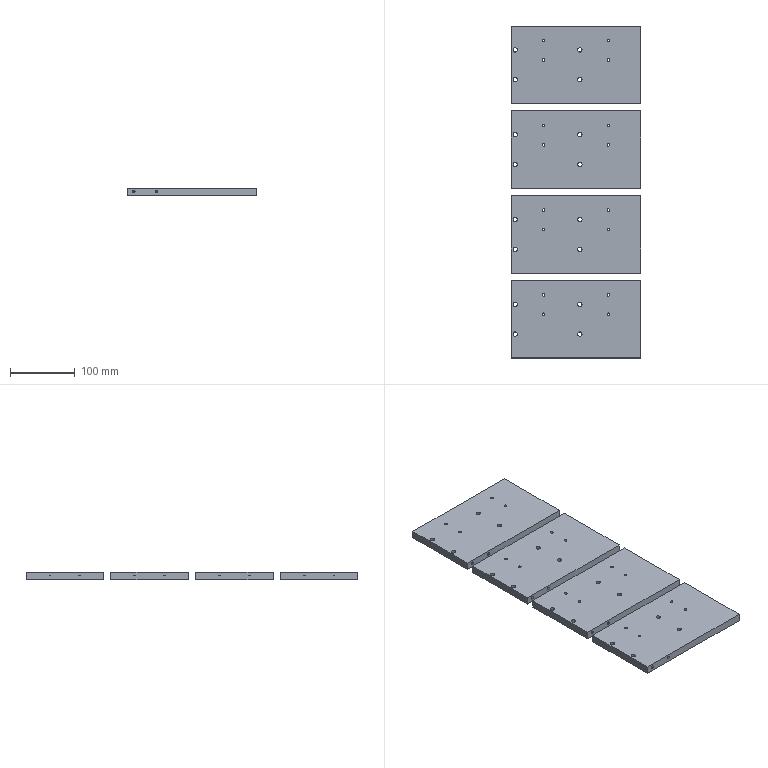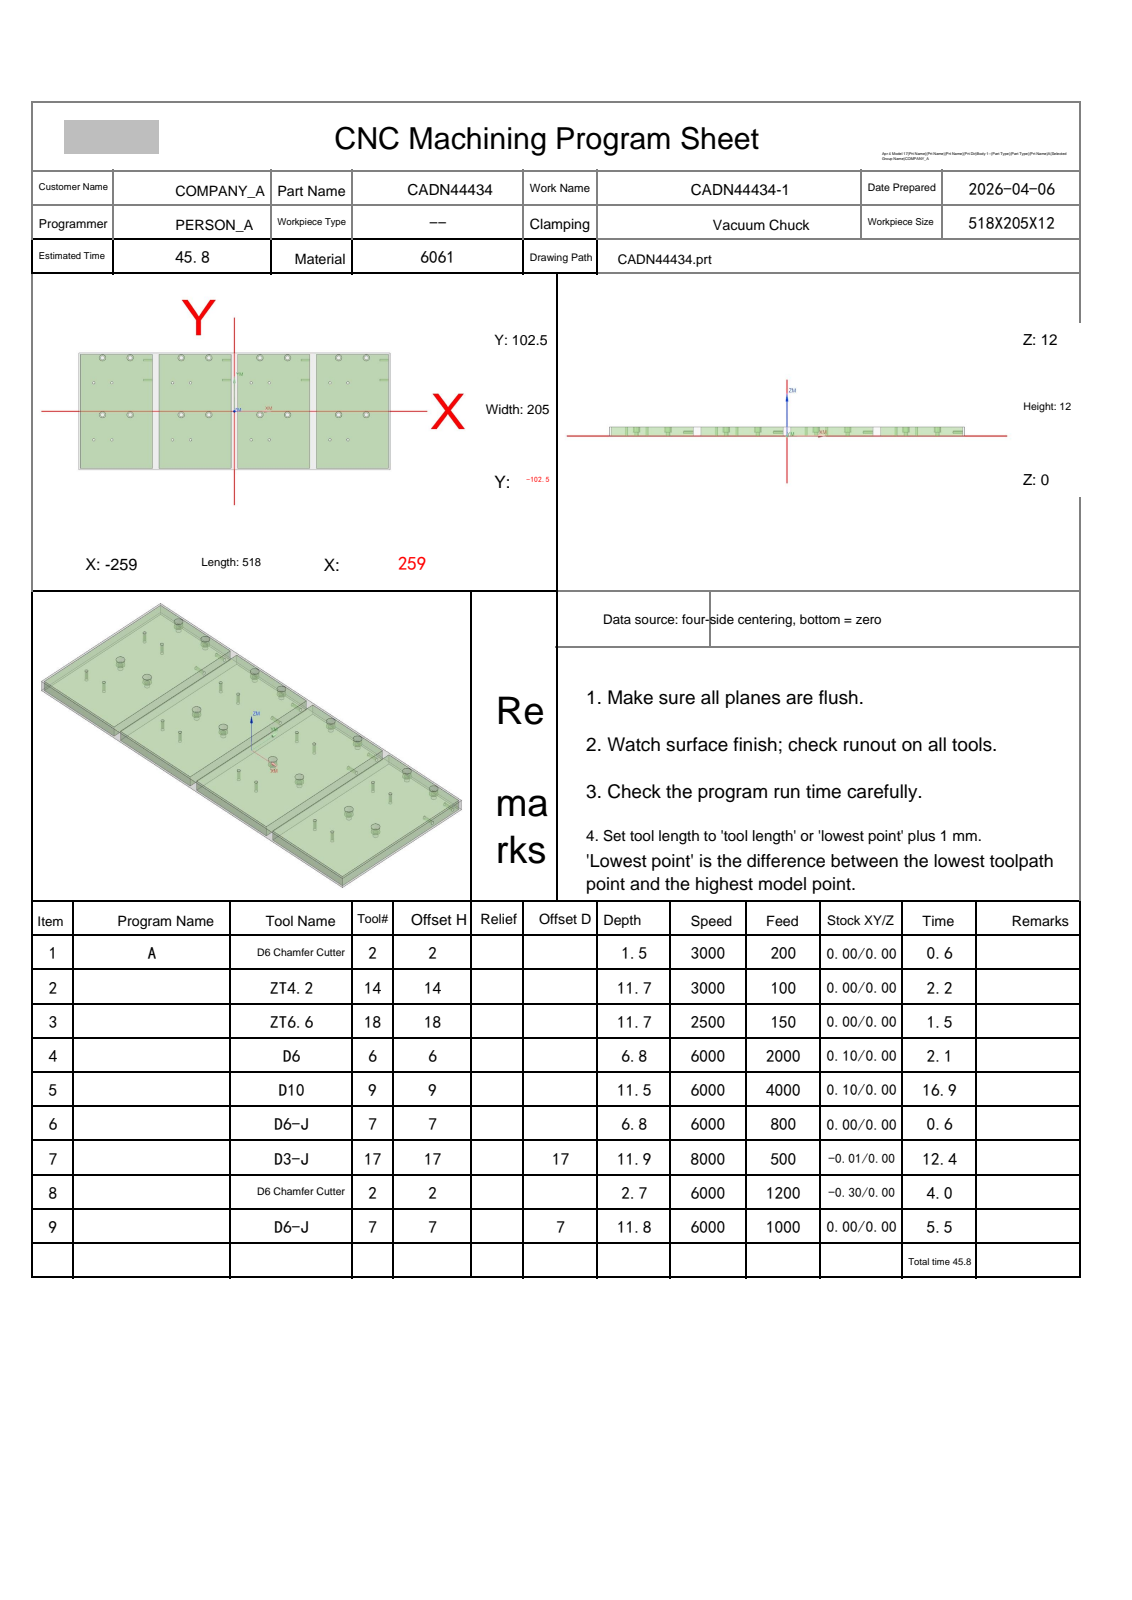NC program | NX | posted by the shop | part box 200 x 513 x 12 mm
Lines 1644 to 2457 of 7719:
N7 T17 M06
(D3-J  D=3. R=0. H=17 ce=-0.01 di=0.00)
G00 G90 G54 X28.521 Y-50.146 M03 S8000
G43 H17 Z32.
M08
Z12.5
G01 X28.543 Y-50.074 Z12.496 F500.
Y-49.926 Z12.488
X28.491 Y-49.757 Z12.479
X28.387 Y-49.613 Z12.47
X28.243 Y-49.509 Z12.46
X28.074 Y-49.457 Z12.451
X27.926 Z12.443
X27.757 Y-49.509 Z12.434
X27.613 Y-49.613 Z12.425
X27.509 Y-49.757 Z12.416
X27.457 Y-49.926 Z12.406
Y-50.074 Z12.398
X27.505 Y-50.235 Z12.39
X27.6 Y-50.375 Z12.381
X27.733 Y-50.478 Z12.372
X27.891 Y-50.537 Z12.363
X28.074 Y-50.543 Z12.354
X28.243 Y-50.491 Z12.344
X28.387 Y-50.387 Z12.335
X28.491 Y-50.243 Z12.326
X28.543 Y-50.074 Z12.316
Y-49.926 Z12.309
X28.491 Y-49.757 Z12.299
X28.387 Y-49.613 Z12.29
X28.243 Y-49.509 Z12.281
X28.074 Y-49.457 Z12.271
X27.926 Z12.264
X27.757 Y-49.509 Z12.254
X27.613 Y-49.613 Z12.245
X27.509 Y-49.757 Z12.236
X27.457 Y-49.926 Z12.227
Y-50.074 Z12.219
X27.505 Y-50.235 Z12.21
X27.6 Y-50.375 Z12.201
X27.733 Y-50.478 Z12.192
X27.891 Y-50.537 Z12.184
X28.074 Y-50.543 Z12.174
X28.243 Y-50.491 Z12.165
X28.387 Y-50.387 Z12.155
X28.491 Y-50.243 Z12.146
X28.543 Y-50.074 Z12.137
Y-49.926 Z12.129
X28.491 Y-49.757 Z12.12
X28.387 Y-49.613 Z12.11
X28.243 Y-49.509 Z12.101
X28.074 Y-49.457 Z12.092
X27.926 Z12.084
X27.757 Y-49.509 Z12.075
X27.613 Y-49.613 Z12.066
X27.509 Y-49.757 Z12.056
X27.457 Y-49.926 Z12.047
Y-50.074 Z12.039
X27.505 Y-50.235 Z12.03
X27.6 Y-50.375 Z12.022
X27.733 Y-50.478 Z12.013
X27.891 Y-50.537 Z12.004
X27.965 Y-50.542 Z12.
G41 D17
X28. Y-50.577
G03 X28.577 Y-50. Z11.926 I0.0 J.577
X28. Y-49.423 Z11.852 I-.577 J0.0
X27.423 Y-50. Z11.778 I0.0 J-.577
X28. Y-50.577 Z11.704 I.577 J0.0
X28.577 Y-50. Z11.63 I0.0 J.577
X28. Y-49.423 Z11.556 I-.577 J0.0
X27.423 Y-50. Z11.482 I0.0 J-.577
X28. Y-50.577 Z11.408 I.577 J0.0
X28.577 Y-50. Z11.333 I0.0 J.577
X28. Y-49.423 Z11.259 I-.577 J0.0
X27.423 Y-50. Z11.185 I0.0 J-.577
X28. Y-50.577 Z11.111 I.577 J0.0
X28.577 Y-50. Z11.037 I0.0 J.577
X28. Y-49.423 Z10.963 I-.577 J0.0
X27.423 Y-50. Z10.889 I0.0 J-.577
X28. Y-50.577 Z10.815 I.577 J0.0
X28.577 Y-50. Z10.741 I0.0 J.577
X28. Y-49.423 Z10.667 I-.577 J0.0
X27.423 Y-50. Z10.593 I0.0 J-.577
X28. Y-50.577 Z10.519 I.577 J0.0
X28.577 Y-50. Z10.445 I0.0 J.577
X28. Y-49.423 Z10.371 I-.577 J0.0
X27.423 Y-50. Z10.297 I0.0 J-.577
X28. Y-50.577 Z10.223 I.577 J0.0
X28.577 Y-50. Z10.148 I0.0 J.577
X28. Y-49.423 Z10.074 I-.577 J0.0
X27.423 Y-50. Z10. I0.0 J-.577
X28. Y-50.577 Z9.926 I.577 J0.0
X28.577 Y-50. Z9.852 I0.0 J.577
X28. Y-49.423 Z9.778 I-.577 J0.0
X27.423 Y-50. Z9.704 I0.0 J-.577
X28. Y-50.577 Z9.63 I.577 J0.0
X28.577 Y-50. Z9.556 I0.0 J.577
X28. Y-49.423 Z9.482 I-.577 J0.0
X27.423 Y-50. Z9.408 I0.0 J-.577
X28. Y-50.577 Z9.334 I.577 J0.0
X28.577 Y-50. Z9.26 I0.0 J.577
X28. Y-49.423 Z9.186 I-.577 J0.0
X27.423 Y-50. Z9.112 I0.0 J-.577
X28. Y-50.577 Z9.038 I.577 J0.0
X28.577 Y-50. Z8.963 I0.0 J.577
X28. Y-49.423 Z8.889 I-.577 J0.0
X27.423 Y-50. Z8.815 I0.0 J-.577
X28. Y-50.577 Z8.741 I.577 J0.0
X28.577 Y-50. Z8.667 I0.0 J.577
X28. Y-49.423 Z8.593 I-.577 J0.0
X27.423 Y-50. Z8.519 I0.0 J-.577
X28. Y-50.577 Z8.445 I.577 J0.0
X28.577 Y-50. Z8.371 I0.0 J.577
X28. Y-49.423 Z8.297 I-.577 J0.0
X27.423 Y-50. Z8.223 I0.0 J-.577
X28. Y-50.577 Z8.149 I.577 J0.0
X28.577 Y-50. Z8.075 I0.0 J.577
X28. Y-49.423 Z8.001 I-.577 J0.0
X27.423 Y-50. Z7.927 I0.0 J-.577
X28. Y-50.577 Z7.853 I.577 J0.0
X28.577 Y-50. Z7.778 I0.0 J.577
X28. Y-49.423 Z7.704 I-.577 J0.0
X27.423 Y-50. Z7.63 I0.0 J-.577
X28. Y-50.577 Z7.556 I.577 J0.0
X28.577 Y-50. Z7.482 I0.0 J.577
X28. Y-49.423 Z7.408 I-.577 J0.0
X27.423 Y-50. Z7.334 I0.0 J-.577
X28. Y-50.577 Z7.26 I.577 J0.0
X28.577 Y-50. Z7.186 I0.0 J.577
X28. Y-49.423 Z7.112 I-.577 J0.0
X27.423 Y-50. Z7.038 I0.0 J-.577
X28. Y-50.577 Z6.964 I.577 J0.0
X28.577 Y-50. Z6.89 I0.0 J.577
X28. Y-49.423 Z6.816 I-.577 J0.0
X27.423 Y-50. Z6.742 I0.0 J-.577
X28. Y-50.577 Z6.668 I.577 J0.0
X28.577 Y-50. Z6.593 I0.0 J.577
X28. Y-49.423 Z6.519 I-.577 J0.0
X27.423 Y-50. Z6.445 I0.0 J-.577
X28. Y-50.577 Z6.371 I.577 J0.0
X28.577 Y-50. Z6.297 I0.0 J.577
X28. Y-49.423 Z6.223 I-.577 J0.0
X27.423 Y-50. Z6.149 I0.0 J-.577
X28. Y-50.577 Z6.075 I.577 J0.0
X28.577 Y-50. Z6.001 I0.0 J.577
X28. Y-49.423 Z5.927 I-.577 J0.0
X27.423 Y-50. Z5.853 I0.0 J-.577
X28. Y-50.577 Z5.779 I.577 J0.0
X28.577 Y-50. Z5.705 I0.0 J.577
X28. Y-49.423 Z5.631 I-.577 J0.0
X27.423 Y-50. Z5.557 I0.0 J-.577
X28. Y-50.577 Z5.483 I.577 J0.0
X28.577 Y-50. Z5.408 I0.0 J.577
X28. Y-49.423 Z5.334 I-.577 J0.0
X27.423 Y-50. Z5.26 I0.0 J-.577
X28. Y-50.577 Z5.186 I.577 J0.0
X28.577 Y-50. Z5.112 I0.0 J.577
X28. Y-49.423 Z5.038 I-.577 J0.0
X27.423 Y-50. Z4.964 I0.0 J-.577
X28. Y-50.577 Z4.89 I.577 J0.0
X28.577 Y-50. Z4.816 I0.0 J.577
X28. Y-49.423 Z4.742 I-.577 J0.0
X27.423 Y-50. Z4.668 I0.0 J-.577
X28. Y-50.577 Z4.594 I.577 J0.0
X28.577 Y-50. Z4.52 I0.0 J.577
X28. Y-49.423 Z4.446 I-.577 J0.0
X27.423 Y-50. Z4.372 I0.0 J-.577
X28. Y-50.577 Z4.298 I.577 J0.0
X28.577 Y-50. Z4.223 I0.0 J.577
X28. Y-49.423 Z4.149 I-.577 J0.0
X27.423 Y-50. Z4.075 I0.0 J-.577
X28. Y-50.577 Z4.001 I.577 J0.0
X28.577 Y-50. Z3.927 I0.0 J.577
X28. Y-49.423 Z3.853 I-.577 J0.0
X27.423 Y-50. Z3.779 I0.0 J-.577
X28. Y-50.577 Z3.705 I.577 J0.0
X28.577 Y-50. Z3.631 I0.0 J.577
X28. Y-49.423 Z3.557 I-.577 J0.0
X27.423 Y-50. Z3.483 I0.0 J-.577
X28. Y-50.577 Z3.409 I.577 J0.0
X28.577 Y-50. Z3.335 I0.0 J.577
X28. Y-49.423 Z3.261 I-.577 J0.0
X27.423 Y-50. Z3.187 I0.0 J-.577
X28. Y-50.577 Z3.113 I.577 J0.0
X28.577 Y-50. Z3.038 I0.0 J.577
X28. Y-49.423 Z2.964 I-.577 J0.0
X27.423 Y-50. Z2.89 I0.0 J-.577
X28. Y-50.577 Z2.816 I.577 J0.0
X28.577 Y-50. Z2.742 I0.0 J.577
X28. Y-49.423 Z2.668 I-.577 J0.0
X27.423 Y-50. Z2.594 I0.0 J-.577
X28. Y-50.577 Z2.52 I.577 J0.0
X28.577 Y-50. Z2.446 I0.0 J.577
X28. Y-49.423 Z2.372 I-.577 J0.0
X27.423 Y-50. Z2.298 I0.0 J-.577
X28. Y-50.577 Z2.224 I.577 J0.0
X28.577 Y-50. Z2.15 I0.0 J.577
X28. Y-49.423 Z2.076 I-.577 J0.0
X27.423 Y-50. Z2.002 I0.0 J-.577
X28. Y-50.577 Z1.928 I.577 J0.0
X28.577 Y-50. Z1.853 I0.0 J.577
X28. Y-49.423 Z1.779 I-.577 J0.0
X27.423 Y-50. Z1.705 I0.0 J-.577
X28. Y-50.577 Z1.631 I.577 J0.0
X28.577 Y-50. Z1.557 I0.0 J.577
X28. Y-49.423 Z1.483 I-.577 J0.0
X27.423 Y-50. Z1.409 I0.0 J-.577
X28. Y-50.577 Z1.335 I.577 J0.0
X28.577 Y-50. Z1.261 I0.0 J.577
X28. Y-49.423 Z1.187 I-.577 J0.0
X27.423 Y-50. Z1.113 I0.0 J-.577
X28. Y-50.577 Z1.039 I.577 J0.0
X28.577 Y-50. Z.965 I0.0 J.577
X28. Y-49.423 Z.891 I-.577 J0.0
X27.423 Y-50. Z.817 I0.0 J-.577
X28. Y-50.577 Z.743 I.577 J0.0
X28.577 Y-50. Z.668 I0.0 J.577
X28. Y-49.423 Z.594 I-.577 J0.0
X27.423 Y-50. Z.52 I0.0 J-.577
X28. Y-50.577 Z.446 I.577 J0.0
X28.577 Y-50. Z.372 I0.0 J.577
X28. Y-49.423 Z.298 I-.577 J0.0
X27.423 Y-50. Z.224 I0.0 J-.577
X28. Y-50.577 Z.15 I.577 J0.0
X28.577 Y-50. I0.0 J.577
X28. Y-49.423 I-.577 J0.0
X27.423 Y-50. I0.0 J-.577
X28. Y-50.577 I.577 J0.0
X28.369 Y-50.444 I0.0 J.577
G01 X28.388 Y-50.424
X28.391 Y-50.396
X28.375 Y-50.373
G40 X28.343 Y-50.335
Z1.15
G00 Z32.
X58.521 Y-50.146
Z12.5
G01 X58.543 Y-50.074 Z12.496
Y-49.926 Z12.488
X58.491 Y-49.757 Z12.479
X58.387 Y-49.613 Z12.47
X58.243 Y-49.509 Z12.46
X58.074 Y-49.457 Z12.451
X57.926 Z12.443
X57.757 Y-49.509 Z12.434
X57.613 Y-49.613 Z12.425
X57.509 Y-49.757 Z12.416
X57.457 Y-49.926 Z12.406
Y-50.074 Z12.398
X57.505 Y-50.235 Z12.39
X57.6 Y-50.375 Z12.381
X57.733 Y-50.478 Z12.372
X57.891 Y-50.537 Z12.363
X58.074 Y-50.543 Z12.354
X58.243 Y-50.491 Z12.344
X58.387 Y-50.387 Z12.335
X58.491 Y-50.243 Z12.326
X58.543 Y-50.074 Z12.316
Y-49.926 Z12.309
X58.491 Y-49.757 Z12.299
X58.387 Y-49.613 Z12.29
X58.243 Y-49.509 Z12.281
X58.074 Y-49.457 Z12.271
X57.926 Z12.264
X57.757 Y-49.509 Z12.254
X57.613 Y-49.613 Z12.245
X57.509 Y-49.757 Z12.236
X57.457 Y-49.926 Z12.227
Y-50.074 Z12.219
X57.505 Y-50.235 Z12.21
X57.6 Y-50.375 Z12.201
X57.733 Y-50.478 Z12.192
X57.891 Y-50.537 Z12.184
X58.074 Y-50.543 Z12.174
X58.243 Y-50.491 Z12.165
X58.387 Y-50.387 Z12.155
X58.491 Y-50.243 Z12.146
X58.543 Y-50.074 Z12.137
Y-49.926 Z12.129
X58.491 Y-49.757 Z12.12
X58.387 Y-49.613 Z12.11
X58.243 Y-49.509 Z12.101
X58.074 Y-49.457 Z12.092
X57.926 Z12.084
X57.757 Y-49.509 Z12.075
X57.613 Y-49.613 Z12.066
X57.509 Y-49.757 Z12.056
X57.457 Y-49.926 Z12.047
Y-50.074 Z12.039
X57.505 Y-50.235 Z12.03
X57.6 Y-50.375 Z12.022
X57.733 Y-50.478 Z12.013
X57.891 Y-50.537 Z12.004
X57.965 Y-50.542 Z12.
G41 D17
X58. Y-50.577
G03 X58.577 Y-50. Z11.926 I0.0 J.577
X58. Y-49.423 Z11.852 I-.577 J0.0
X57.423 Y-50. Z11.778 I0.0 J-.577
X58. Y-50.577 Z11.704 I.577 J0.0
X58.577 Y-50. Z11.63 I0.0 J.577
X58. Y-49.423 Z11.556 I-.577 J0.0
X57.423 Y-50. Z11.482 I0.0 J-.577
X58. Y-50.577 Z11.408 I.577 J0.0
X58.577 Y-50. Z11.333 I0.0 J.577
X58. Y-49.423 Z11.259 I-.577 J0.0
X57.423 Y-50. Z11.185 I0.0 J-.577
X58. Y-50.577 Z11.111 I.577 J0.0
X58.577 Y-50. Z11.037 I0.0 J.577
X58. Y-49.423 Z10.963 I-.577 J0.0
X57.423 Y-50. Z10.889 I0.0 J-.577
X58. Y-50.577 Z10.815 I.577 J0.0
X58.577 Y-50. Z10.741 I0.0 J.577
X58. Y-49.423 Z10.667 I-.577 J0.0
X57.423 Y-50. Z10.593 I0.0 J-.577
X58. Y-50.577 Z10.519 I.577 J0.0
X58.577 Y-50. Z10.445 I0.0 J.577
X58. Y-49.423 Z10.371 I-.577 J0.0
X57.423 Y-50. Z10.297 I0.0 J-.577
X58. Y-50.577 Z10.223 I.577 J0.0
X58.577 Y-50. Z10.148 I0.0 J.577
X58. Y-49.423 Z10.074 I-.577 J0.0
X57.423 Y-50. Z10. I0.0 J-.577
X58. Y-50.577 Z9.926 I.577 J0.0
X58.577 Y-50. Z9.852 I0.0 J.577
X58. Y-49.423 Z9.778 I-.577 J0.0
X57.423 Y-50. Z9.704 I0.0 J-.577
X58. Y-50.577 Z9.63 I.577 J0.0
X58.577 Y-50. Z9.556 I0.0 J.577
X58. Y-49.423 Z9.482 I-.577 J0.0
X57.423 Y-50. Z9.408 I0.0 J-.577
X58. Y-50.577 Z9.334 I.577 J0.0
X58.577 Y-50. Z9.26 I0.0 J.577
X58. Y-49.423 Z9.186 I-.577 J0.0
X57.423 Y-50. Z9.112 I0.0 J-.577
X58. Y-50.577 Z9.038 I.577 J0.0
X58.577 Y-50. Z8.963 I0.0 J.577
X58. Y-49.423 Z8.889 I-.577 J0.0
X57.423 Y-50. Z8.815 I0.0 J-.577
X58. Y-50.577 Z8.741 I.577 J0.0
X58.577 Y-50. Z8.667 I0.0 J.577
X58. Y-49.423 Z8.593 I-.577 J0.0
X57.423 Y-50. Z8.519 I0.0 J-.577
X58. Y-50.577 Z8.445 I.577 J0.0
X58.577 Y-50. Z8.371 I0.0 J.577
X58. Y-49.423 Z8.297 I-.577 J0.0
X57.423 Y-50. Z8.223 I0.0 J-.577
X58. Y-50.577 Z8.149 I.577 J0.0
X58.577 Y-50. Z8.075 I0.0 J.577
X58. Y-49.423 Z8.001 I-.577 J0.0
X57.423 Y-50. Z7.927 I0.0 J-.577
X58. Y-50.577 Z7.853 I.577 J0.0
X58.577 Y-50. Z7.778 I0.0 J.577
X58. Y-49.423 Z7.704 I-.577 J0.0
X57.423 Y-50. Z7.63 I0.0 J-.577
X58. Y-50.577 Z7.556 I.577 J0.0
X58.577 Y-50. Z7.482 I0.0 J.577
X58. Y-49.423 Z7.408 I-.577 J0.0
X57.423 Y-50. Z7.334 I0.0 J-.577
X58. Y-50.577 Z7.26 I.577 J0.0
X58.577 Y-50. Z7.186 I0.0 J.577
X58. Y-49.423 Z7.112 I-.577 J0.0
X57.423 Y-50. Z7.038 I0.0 J-.577
X58. Y-50.577 Z6.964 I.577 J0.0
X58.577 Y-50. Z6.89 I0.0 J.577
X58. Y-49.423 Z6.816 I-.577 J0.0
X57.423 Y-50. Z6.742 I0.0 J-.577
X58. Y-50.577 Z6.668 I.577 J0.0
X58.577 Y-50. Z6.593 I0.0 J.577
X58. Y-49.423 Z6.519 I-.577 J0.0
X57.423 Y-50. Z6.445 I0.0 J-.577
X58. Y-50.577 Z6.371 I.577 J0.0
X58.577 Y-50. Z6.297 I0.0 J.577
X58. Y-49.423 Z6.223 I-.577 J0.0
X57.423 Y-50. Z6.149 I0.0 J-.577
X58. Y-50.577 Z6.075 I.577 J0.0
X58.577 Y-50. Z6.001 I0.0 J.577
X58. Y-49.423 Z5.927 I-.577 J0.0
X57.423 Y-50. Z5.853 I0.0 J-.577
X58. Y-50.577 Z5.779 I.577 J0.0
X58.577 Y-50. Z5.705 I0.0 J.577
X58. Y-49.423 Z5.631 I-.577 J0.0
X57.423 Y-50. Z5.557 I0.0 J-.577
X58. Y-50.577 Z5.483 I.577 J0.0
X58.577 Y-50. Z5.408 I0.0 J.577
X58. Y-49.423 Z5.334 I-.577 J0.0
X57.423 Y-50. Z5.26 I0.0 J-.577
X58. Y-50.577 Z5.186 I.577 J0.0
X58.577 Y-50. Z5.112 I0.0 J.577
X58. Y-49.423 Z5.038 I-.577 J0.0
X57.423 Y-50. Z4.964 I0.0 J-.577
X58. Y-50.577 Z4.89 I.577 J0.0
X58.577 Y-50. Z4.816 I0.0 J.577
X58. Y-49.423 Z4.742 I-.577 J0.0
X57.423 Y-50. Z4.668 I0.0 J-.577
X58. Y-50.577 Z4.594 I.577 J0.0
X58.577 Y-50. Z4.52 I0.0 J.577
X58. Y-49.423 Z4.446 I-.577 J0.0
X57.423 Y-50. Z4.372 I0.0 J-.577
X58. Y-50.577 Z4.298 I.577 J0.0
X58.577 Y-50. Z4.223 I0.0 J.577
X58. Y-49.423 Z4.149 I-.577 J0.0
X57.423 Y-50. Z4.075 I0.0 J-.577
X58. Y-50.577 Z4.001 I.577 J0.0
X58.577 Y-50. Z3.927 I0.0 J.577
X58. Y-49.423 Z3.853 I-.577 J0.0
X57.423 Y-50. Z3.779 I0.0 J-.577
X58. Y-50.577 Z3.705 I.577 J0.0
X58.577 Y-50. Z3.631 I0.0 J.577
X58. Y-49.423 Z3.557 I-.577 J0.0
X57.423 Y-50. Z3.483 I0.0 J-.577
X58. Y-50.577 Z3.409 I.577 J0.0
X58.577 Y-50. Z3.335 I0.0 J.577
X58. Y-49.423 Z3.261 I-.577 J0.0
X57.423 Y-50. Z3.187 I0.0 J-.577
X58. Y-50.577 Z3.113 I.577 J0.0
X58.577 Y-50. Z3.038 I0.0 J.577
X58. Y-49.423 Z2.964 I-.577 J0.0
X57.423 Y-50. Z2.89 I0.0 J-.577
X58. Y-50.577 Z2.816 I.577 J0.0
X58.577 Y-50. Z2.742 I0.0 J.577
X58. Y-49.423 Z2.668 I-.577 J0.0
X57.423 Y-50. Z2.594 I0.0 J-.577
X58. Y-50.577 Z2.52 I.577 J0.0
X58.577 Y-50. Z2.446 I0.0 J.577
X58. Y-49.423 Z2.372 I-.577 J0.0
X57.423 Y-50. Z2.298 I0.0 J-.577
X58. Y-50.577 Z2.224 I.577 J0.0
X58.577 Y-50. Z2.15 I0.0 J.577
X58. Y-49.423 Z2.076 I-.577 J0.0
X57.423 Y-50. Z2.002 I0.0 J-.577
X58. Y-50.577 Z1.928 I.577 J0.0
X58.577 Y-50. Z1.853 I0.0 J.577
X58. Y-49.423 Z1.779 I-.577 J0.0
X57.423 Y-50. Z1.705 I0.0 J-.577
X58. Y-50.577 Z1.631 I.577 J0.0
X58.577 Y-50. Z1.557 I0.0 J.577
X58. Y-49.423 Z1.483 I-.577 J0.0
X57.423 Y-50. Z1.409 I0.0 J-.577
X58. Y-50.577 Z1.335 I.577 J0.0
X58.577 Y-50. Z1.261 I0.0 J.577
X58. Y-49.423 Z1.187 I-.577 J0.0
X57.423 Y-50. Z1.113 I0.0 J-.577
X58. Y-50.577 Z1.039 I.577 J0.0
X58.577 Y-50. Z.965 I0.0 J.577
X58. Y-49.423 Z.891 I-.577 J0.0
X57.423 Y-50. Z.817 I0.0 J-.577
X58. Y-50.577 Z.743 I.577 J0.0
X58.577 Y-50. Z.668 I0.0 J.577
X58. Y-49.423 Z.594 I-.577 J0.0
X57.423 Y-50. Z.52 I0.0 J-.577
X58. Y-50.577 Z.446 I.577 J0.0
X58.577 Y-50. Z.372 I0.0 J.577
X58. Y-49.423 Z.298 I-.577 J0.0
X57.423 Y-50. Z.224 I0.0 J-.577
X58. Y-50.577 Z.15 I.577 J0.0
X58.577 Y-50. I0.0 J.577
X58. Y-49.423 I-.577 J0.0
X57.423 Y-50. I0.0 J-.577
X58. Y-50.577 I.577 J0.0
X58.369 Y-50.444 I0.0 J.577
G01 X58.388 Y-50.424
X58.391 Y-50.396
X58.375 Y-50.373
G40 X58.343 Y-50.335
Z1.15
G00 Z32.
X159.521 Y-50.146
Z12.5
G01 X159.543 Y-50.074 Z12.496
Y-49.926 Z12.488
X159.491 Y-49.757 Z12.479
X159.387 Y-49.613 Z12.47
X159.243 Y-49.509 Z12.46
X159.074 Y-49.457 Z12.451
X158.926 Z12.443
X158.757 Y-49.509 Z12.434
X158.613 Y-49.613 Z12.425
X158.509 Y-49.757 Z12.416
X158.457 Y-49.926 Z12.406
Y-50.074 Z12.398
X158.505 Y-50.235 Z12.39
X158.6 Y-50.375 Z12.381
X158.733 Y-50.478 Z12.372
X158.891 Y-50.537 Z12.363
X159.074 Y-50.543 Z12.354
X159.243 Y-50.491 Z12.344
X159.387 Y-50.387 Z12.335
X159.491 Y-50.243 Z12.326
X159.543 Y-50.074 Z12.316
Y-49.926 Z12.309
X159.491 Y-49.757 Z12.299
X159.387 Y-49.613 Z12.29
X159.243 Y-49.509 Z12.281
X159.074 Y-49.457 Z12.271
X158.926 Z12.264
X158.757 Y-49.509 Z12.254
X158.613 Y-49.613 Z12.245
X158.509 Y-49.757 Z12.236
X158.457 Y-49.926 Z12.227
Y-50.074 Z12.219
X158.505 Y-50.235 Z12.21
X158.6 Y-50.375 Z12.201
X158.733 Y-50.478 Z12.192
X158.891 Y-50.537 Z12.184
X159.074 Y-50.543 Z12.174
X159.243 Y-50.491 Z12.165
X159.387 Y-50.387 Z12.155
X159.491 Y-50.243 Z12.146
X159.543 Y-50.074 Z12.137
Y-49.926 Z12.129
X159.491 Y-49.757 Z12.12
X159.387 Y-49.613 Z12.11
X159.243 Y-49.509 Z12.101
X159.074 Y-49.457 Z12.092
X158.926 Z12.084
X158.757 Y-49.509 Z12.075
X158.613 Y-49.613 Z12.066
X158.509 Y-49.757 Z12.056
X158.457 Y-49.926 Z12.047
Y-50.074 Z12.039
X158.505 Y-50.235 Z12.03
X158.6 Y-50.375 Z12.022
X158.733 Y-50.478 Z12.013
X158.891 Y-50.537 Z12.004
X158.965 Y-50.542 Z12.
G41 D17
X159. Y-50.577
G03 X159.577 Y-50. Z11.926 I0.0 J.577
X159. Y-49.423 Z11.852 I-.577 J0.0
X158.423 Y-50. Z11.778 I0.0 J-.577
X159. Y-50.577 Z11.704 I.577 J0.0
X159.577 Y-50. Z11.63 I0.0 J.577
X159. Y-49.423 Z11.556 I-.577 J0.0
X158.423 Y-50. Z11.482 I0.0 J-.577
X159. Y-50.577 Z11.408 I.577 J0.0
X159.577 Y-50. Z11.333 I0.0 J.577
X159. Y-49.423 Z11.259 I-.577 J0.0
X158.423 Y-50. Z11.185 I0.0 J-.577
X159. Y-50.577 Z11.111 I.577 J0.0
X159.577 Y-50. Z11.037 I0.0 J.577
X159. Y-49.423 Z10.963 I-.577 J0.0
X158.423 Y-50. Z10.889 I0.0 J-.577
X159. Y-50.577 Z10.815 I.577 J0.0
X159.577 Y-50. Z10.741 I0.0 J.577
X159. Y-49.423 Z10.667 I-.577 J0.0
X158.423 Y-50. Z10.593 I0.0 J-.577
X159. Y-50.577 Z10.519 I.577 J0.0
X159.577 Y-50. Z10.445 I0.0 J.577
X159. Y-49.423 Z10.371 I-.577 J0.0
X158.423 Y-50. Z10.297 I0.0 J-.577
X159. Y-50.577 Z10.223 I.577 J0.0
X159.577 Y-50. Z10.148 I0.0 J.577
X159. Y-49.423 Z10.074 I-.577 J0.0
X158.423 Y-50. Z10. I0.0 J-.577
X159. Y-50.577 Z9.926 I.577 J0.0
X159.577 Y-50. Z9.852 I0.0 J.577
X159. Y-49.423 Z9.778 I-.577 J0.0
X158.423 Y-50. Z9.704 I0.0 J-.577
X159. Y-50.577 Z9.63 I.577 J0.0
X159.577 Y-50. Z9.556 I0.0 J.577
X159. Y-49.423 Z9.482 I-.577 J0.0
X158.423 Y-50. Z9.408 I0.0 J-.577
X159. Y-50.577 Z9.334 I.577 J0.0
X159.577 Y-50. Z9.26 I0.0 J.577
X159. Y-49.423 Z9.186 I-.577 J0.0
X158.423 Y-50. Z9.112 I0.0 J-.577
X159. Y-50.577 Z9.038 I.577 J0.0
X159.577 Y-50. Z8.963 I0.0 J.577
X159. Y-49.423 Z8.889 I-.577 J0.0
X158.423 Y-50. Z8.815 I0.0 J-.577
X159. Y-50.577 Z8.741 I.577 J0.0
X159.577 Y-50. Z8.667 I0.0 J.577
X159. Y-49.423 Z8.593 I-.577 J0.0
X158.423 Y-50. Z8.519 I0.0 J-.577
X159. Y-50.577 Z8.445 I.577 J0.0
X159.577 Y-50. Z8.371 I0.0 J.577
X159. Y-49.423 Z8.297 I-.577 J0.0
X158.423 Y-50. Z8.223 I0.0 J-.577
X159. Y-50.577 Z8.149 I.577 J0.0
X159.577 Y-50. Z8.075 I0.0 J.577
X159. Y-49.423 Z8.001 I-.577 J0.0
X158.423 Y-50. Z7.927 I0.0 J-.577
X159. Y-50.577 Z7.853 I.577 J0.0
X159.577 Y-50. Z7.778 I0.0 J.577
X159. Y-49.423 Z7.704 I-.577 J0.0
X158.423 Y-50. Z7.63 I0.0 J-.577
X159. Y-50.577 Z7.556 I.577 J0.0
X159.577 Y-50. Z7.482 I0.0 J.577
X159. Y-49.423 Z7.408 I-.577 J0.0
X158.423 Y-50. Z7.334 I0.0 J-.577
X159. Y-50.577 Z7.26 I.577 J0.0
X159.577 Y-50. Z7.186 I0.0 J.577
X159. Y-49.423 Z7.112 I-.577 J0.0
X158.423 Y-50. Z7.038 I0.0 J-.577
X159. Y-50.577 Z6.964 I.577 J0.0
X159.577 Y-50. Z6.89 I0.0 J.577
X159. Y-49.423 Z6.816 I-.577 J0.0
X158.423 Y-50. Z6.742 I0.0 J-.577
X159. Y-50.577 Z6.668 I.577 J0.0
X159.577 Y-50. Z6.593 I0.0 J.577
X159. Y-49.423 Z6.519 I-.577 J0.0
X158.423 Y-50. Z6.445 I0.0 J-.577
X159. Y-50.577 Z6.371 I.577 J0.0
X159.577 Y-50. Z6.297 I0.0 J.577
X159. Y-49.423 Z6.223 I-.577 J0.0
X158.423 Y-50. Z6.149 I0.0 J-.577
X159. Y-50.577 Z6.075 I.577 J0.0
X159.577 Y-50. Z6.001 I0.0 J.577
X159. Y-49.423 Z5.927 I-.577 J0.0
X158.423 Y-50. Z5.853 I0.0 J-.577
X159. Y-50.577 Z5.779 I.577 J0.0
X159.577 Y-50. Z5.705 I0.0 J.577
X159. Y-49.423 Z5.631 I-.577 J0.0
X158.423 Y-50. Z5.557 I0.0 J-.577
X159. Y-50.577 Z5.483 I.577 J0.0
X159.577 Y-50. Z5.408 I0.0 J.577
X159. Y-49.423 Z5.334 I-.577 J0.0
X158.423 Y-50. Z5.26 I0.0 J-.577
X159. Y-50.577 Z5.186 I.577 J0.0
X159.577 Y-50. Z5.112 I0.0 J.577
X159. Y-49.423 Z5.038 I-.577 J0.0
X158.423 Y-50. Z4.964 I0.0 J-.577
X159. Y-50.577 Z4.89 I.577 J0.0
X159.577 Y-50. Z4.816 I0.0 J.577
X159. Y-49.423 Z4.742 I-.577 J0.0
X158.423 Y-50. Z4.668 I0.0 J-.577
X159. Y-50.577 Z4.594 I.577 J0.0
X159.577 Y-50. Z4.52 I0.0 J.577
X159. Y-49.423 Z4.446 I-.577 J0.0
X158.423 Y-50. Z4.372 I0.0 J-.577
X159. Y-50.577 Z4.298 I.577 J0.0
X159.577 Y-50. Z4.223 I0.0 J.577
X159. Y-49.423 Z4.149 I-.577 J0.0
X158.423 Y-50. Z4.075 I0.0 J-.577
X159. Y-50.577 Z4.001 I.577 J0.0
X159.577 Y-50. Z3.927 I0.0 J.577
X159. Y-49.423 Z3.853 I-.577 J0.0
X158.423 Y-50. Z3.779 I0.0 J-.577
X159. Y-50.577 Z3.705 I.577 J0.0
X159.577 Y-50. Z3.631 I0.0 J.577
X159. Y-49.423 Z3.557 I-.577 J0.0
X158.423 Y-50. Z3.483 I0.0 J-.577
X159. Y-50.577 Z3.409 I.577 J0.0
X159.577 Y-50. Z3.335 I0.0 J.577
X159. Y-49.423 Z3.261 I-.577 J0.0
X158.423 Y-50. Z3.187 I0.0 J-.577
X159. Y-50.577 Z3.113 I.577 J0.0
X159.577 Y-50. Z3.038 I0.0 J.577
X159. Y-49.423 Z2.964 I-.577 J0.0
X158.423 Y-50. Z2.89 I0.0 J-.577
X159. Y-50.577 Z2.816 I.577 J0.0
X159.577 Y-50. Z2.742 I0.0 J.577
X159. Y-49.423 Z2.668 I-.577 J0.0
X158.423 Y-50. Z2.594 I0.0 J-.577
X159. Y-50.577 Z2.52 I.577 J0.0
X159.577 Y-50. Z2.446 I0.0 J.577
X159. Y-49.423 Z2.372 I-.577 J0.0
X158.423 Y-50. Z2.298 I0.0 J-.577
X159. Y-50.577 Z2.224 I.577 J0.0
X159.577 Y-50. Z2.15 I0.0 J.577
X159. Y-49.423 Z2.076 I-.577 J0.0
X158.423 Y-50. Z2.002 I0.0 J-.577
X159. Y-50.577 Z1.928 I.577 J0.0
X159.577 Y-50. Z1.853 I0.0 J.577
X159. Y-49.423 Z1.779 I-.577 J0.0
X158.423 Y-50. Z1.705 I0.0 J-.577
X159. Y-50.577 Z1.631 I.577 J0.0
X159.577 Y-50. Z1.557 I0.0 J.577
X159. Y-49.423 Z1.483 I-.577 J0.0
X158.423 Y-50. Z1.409 I0.0 J-.577
X159. Y-50.577 Z1.335 I.577 J0.0
X159.577 Y-50. Z1.261 I0.0 J.577
X159. Y-49.423 Z1.187 I-.577 J0.0
X158.423 Y-50. Z1.113 I0.0 J-.577
X159. Y-50.577 Z1.039 I.577 J0.0
X159.577 Y-50. Z.965 I0.0 J.577
X159. Y-49.423 Z.891 I-.577 J0.0
X158.423 Y-50. Z.817 I0.0 J-.577
X159. Y-50.577 Z.743 I.577 J0.0
X159.577 Y-50. Z.668 I0.0 J.577
X159. Y-49.423 Z.594 I-.577 J0.0
X158.423 Y-50. Z.52 I0.0 J-.577
X159. Y-50.577 Z.446 I.577 J0.0
X159.577 Y-50. Z.372 I0.0 J.577
X159. Y-49.423 Z.298 I-.577 J0.0
X158.423 Y-50. Z.224 I0.0 J-.577
X159. Y-50.577 Z.15 I.577 J0.0
X159.577 Y-50. I0.0 J.577
X159. Y-49.423 I-.577 J0.0
X158.423 Y-50. I0.0 J-.577
X159. Y-50.577 I.577 J0.0
X159.369 Y-50.444 I0.0 J.577
G01 X159.388 Y-50.424
X159.391 Y-50.396
X159.375 Y-50.373
G40 X159.343 Y-50.335
Z1.15
G00 Z32.
X189.521 Y-50.146
Z12.5
G01 X189.543 Y-50.074 Z12.496
Y-49.926 Z12.488
X189.491 Y-49.757 Z12.479
X189.387 Y-49.613 Z12.47
X189.243 Y-49.509 Z12.46
X189.074 Y-49.457 Z12.451
X188.926 Z12.443
X188.757 Y-49.509 Z12.434
X188.613 Y-49.613 Z12.425
X188.509 Y-49.757 Z12.416
X188.457 Y-49.926 Z12.406
Y-50.074 Z12.398
X188.505 Y-50.235 Z12.39
X188.6 Y-50.375 Z12.381
X188.733 Y-50.478 Z12.372
X188.891 Y-50.537 Z12.363
X189.074 Y-50.543 Z12.354
X189.243 Y-50.491 Z12.344
X189.387 Y-50.387 Z12.335
X189.491 Y-50.243 Z12.326
X189.543 Y-50.074 Z12.316
Y-49.926 Z12.309
X189.491 Y-49.757 Z12.299
X189.387 Y-49.613 Z12.29
X189.243 Y-49.509 Z12.281
X189.074 Y-49.457 Z12.271
X188.926 Z12.264
X188.757 Y-49.509 Z12.254
X188.613 Y-49.613 Z12.245
X188.509 Y-49.757 Z12.236
X188.457 Y-49.926 Z12.227
Y-50.074 Z12.219
X188.505 Y-50.235 Z12.21
X188.6 Y-50.375 Z12.201
X188.733 Y-50.478 Z12.192
X188.891 Y-50.537 Z12.184
X189.074 Y-50.543 Z12.174
X189.243 Y-50.491 Z12.165
X189.387 Y-50.387 Z12.155
X189.491 Y-50.243 Z12.146
X189.543 Y-50.074 Z12.137
Y-49.926 Z12.129
X189.491 Y-49.757 Z12.12
X189.387 Y-49.613 Z12.11
X189.243 Y-49.509 Z12.101
X189.074 Y-49.457 Z12.092
X188.926 Z12.084
X188.757 Y-49.509 Z12.075
X188.613 Y-49.613 Z12.066
X188.509 Y-49.757 Z12.056
X188.457 Y-49.926 Z12.047
Y-50.074 Z12.039
X188.505 Y-50.235 Z12.03
X188.6 Y-50.375 Z12.022
X188.733 Y-50.478 Z12.013
X188.891 Y-50.537 Z12.004
X188.965 Y-50.542 Z12.
G41 D17
X189. Y-50.577
G03 X189.577 Y-50. Z11.926 I0.0 J.577
X189. Y-49.423 Z11.852 I-.577 J0.0
X188.423 Y-50. Z11.778 I0.0 J-.577
X189. Y-50.577 Z11.704 I.577 J0.0
X189.577 Y-50. Z11.63 I0.0 J.577
X189. Y-49.423 Z11.556 I-.577 J0.0
X188.423 Y-50. Z11.482 I0.0 J-.577
X189. Y-50.577 Z11.408 I.577 J0.0
X189.577 Y-50. Z11.333 I0.0 J.577
X189. Y-49.423 Z11.259 I-.577 J0.0
X188.423 Y-50. Z11.185 I0.0 J-.577
X189. Y-50.577 Z11.111 I.577 J0.0
X189.577 Y-50. Z11.037 I0.0 J.577
X189. Y-49.423 Z10.963 I-.577 J0.0
X188.423 Y-50. Z10.889 I0.0 J-.577
X189. Y-50.577 Z10.815 I.577 J0.0
X189.577 Y-50. Z10.741 I0.0 J.577
X189. Y-49.423 Z10.667 I-.577 J0.0
X188.423 Y-50. Z10.593 I0.0 J-.577
X189. Y-50.577 Z10.519 I.577 J0.0
X189.577 Y-50. Z10.445 I0.0 J.577
X189. Y-49.423 Z10.371 I-.577 J0.0
X188.423 Y-50. Z10.297 I0.0 J-.577
X189. Y-50.577 Z10.223 I.577 J0.0
X189.577 Y-50. Z10.148 I0.0 J.577
X189. Y-49.423 Z10.074 I-.577 J0.0
X188.423 Y-50. Z10. I0.0 J-.577
X189. Y-50.577 Z9.926 I.577 J0.0
X189.577 Y-50. Z9.852 I0.0 J.577
X189. Y-49.423 Z9.778 I-.577 J0.0
X188.423 Y-50. Z9.704 I0.0 J-.577
X189. Y-50.577 Z9.63 I.577 J0.0
X189.577 Y-50. Z9.556 I0.0 J.577
X189. Y-49.423 Z9.482 I-.577 J0.0
X188.423 Y-50. Z9.408 I0.0 J-.577
X189. Y-50.577 Z9.334 I.577 J0.0
X189.577 Y-50. Z9.26 I0.0 J.577
X189. Y-49.423 Z9.186 I-.577 J0.0
X188.423 Y-50. Z9.112 I0.0 J-.577
X189. Y-50.577 Z9.038 I.577 J0.0
X189.577 Y-50. Z8.963 I0.0 J.577
X189. Y-49.423 Z8.889 I-.577 J0.0
X188.423 Y-50. Z8.815 I0.0 J-.577
X189. Y-50.577 Z8.741 I.577 J0.0
X189.577 Y-50. Z8.667 I0.0 J.577
X189. Y-49.423 Z8.593 I-.577 J0.0
X188.423 Y-50. Z8.519 I0.0 J-.577
X189. Y-50.577 Z8.445 I.577 J0.0
X189.577 Y-50. Z8.371 I0.0 J.577
X189. Y-49.423 Z8.297 I-.577 J0.0
X188.423 Y-50. Z8.223 I0.0 J-.577
X189. Y-50.577 Z8.149 I.577 J0.0
X189.577 Y-50. Z8.075 I0.0 J.577